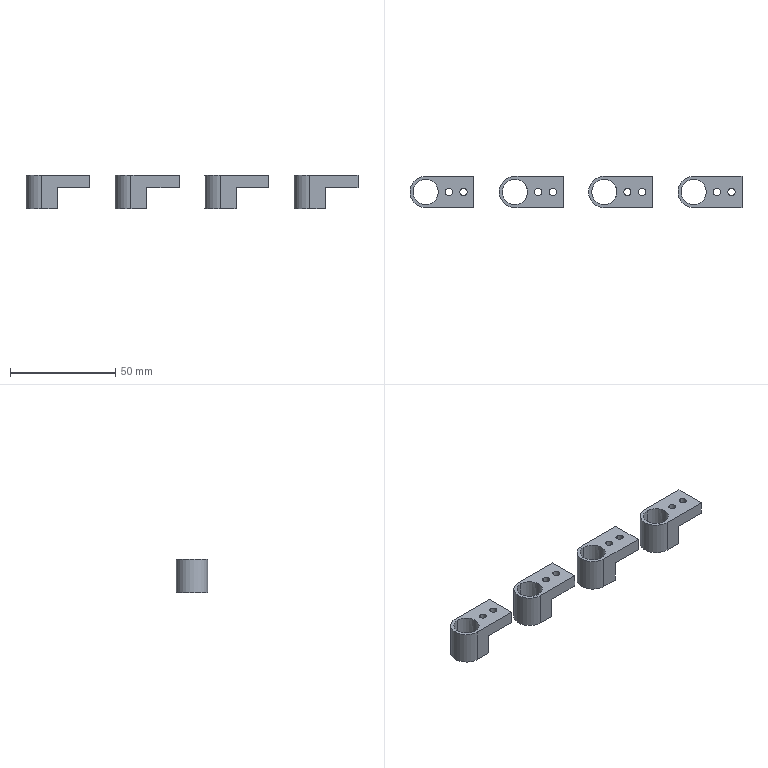NC program | NX | posted with a generic post | part box 158 x 15 x 16 mm
Whole program:
N10 G17 G21 G94 G90
(FLOOR_WALL_COPY , TOOL : D63)
N12 T03 M6
N14 G54
N16 G17 G0 G90 X-34.5 Y0. S6500 M3
N18 G43 Z30. H3
N20 Z6.
N22 G94 G1 Z3. F1500.
N24 X-31.5
N26 X189.5
N28 X192.5
N30 Z6.
N32 G0 Z30.
N34 X-34.5
N36 Z5.
N38 G1 Z2.
N40 X-31.5
N42 X189.5
N44 X192.5
N46 Z5.
N48 G0 Z30.
N50 X-34.5
N52 Z4.
N54 G1 Z1.
N56 X-31.5
N58 X189.5
N60 X192.5
N62 Z4.
N64 G0 Z30.
N66 X-34.5
N68 Z3.
N70 G1 Z0.
N72 X-31.5
N74 X189.5
N76 X192.5
N78 Z3.
N80 G0 Z30.
N82 M5
(FLOOR_WALL_1 , TOOL : D10)
N84 T04 M6
N86 G54
N88 G17 G0 G90 X-4.7 Y-16. S7500 M3
N90 G43 Z30. H4
N92 Z-6.9
N94 G94 G1 Z-9.9 F1000.
N96 Y-13.
N98 Y13. F2500.
N100 X-3.908
N102 Y-13.
N104 X-3.116
N106 Y13.
N108 X-2.324
N110 Y-13.
N112 X-1.532
N114 Y13.
N116 X-0.739
N118 Y-13.
N120 X0.053
N122 Y13.
N124 X0.845
N126 Y-13.
N128 X1.637
N130 Y13.
N132 X2.429
N134 Y-13.
N136 X3.221
N138 Y13.
N140 X4.013
N142 Y-13.
N144 X4.805
N146 Y13.
N148 X5.597
N150 Y-13.
N152 X6.389
N154 Y13.
N156 X7.182
N158 Y-13.
N160 X7.974
N162 Y13.
N164 X8.766
N166 Y-13.
N168 X9.558
N170 Y13.
N172 X10.35
N174 Y-13.
N176 Y-16.
N178 Z-6.9
N180 G0 Z30.
N182 X37.8
N184 Z-6.9
N186 G1 Z-9.9 F1000.
N188 Y-13.
N190 Y13. F2500.
N192 X38.592
N194 Y-13.
N196 X39.384
N198 Y13.
N200 X40.176
N202 Y-13.
N204 X40.968
N206 Y13.
N208 X41.761
N210 Y-13.
N212 X42.553
N214 Y13.
N216 X43.345
N218 Y-13.
N220 X44.137
N222 Y13.
N224 X44.929
N226 Y-13.
N228 X45.721
N230 Y13.
N232 X46.513
N234 Y-13.
N236 X47.305
N238 Y13.
N240 X48.097
N242 Y-13.
N244 X48.889
N246 Y13.
N248 X49.682
N250 Y-13.
N252 X50.474
N254 Y13.
N256 X51.266
N258 Y-13.
N260 X52.058
N262 Y13.
N264 X52.85
N266 Y-13.
N268 Y-16.
N270 Z-6.9
N272 G0 Z30.
N274 X80.3
N276 Z-6.9
N278 G1 Z-9.9 F1000.
N280 Y-13.
N282 Y13. F2500.
N284 X81.092
N286 Y-13.
N288 X81.884
N290 Y13.
N292 X82.676
N294 Y-13.
N296 X83.468
N298 Y13.
N300 X84.261
N302 Y-13.
N304 X85.053
N306 Y13.
N308 X85.845
N310 Y-13.
N312 X86.637
N314 Y13.
N316 X87.429
N318 Y-13.
N320 X88.221
N322 Y13.
N324 X89.013
N326 Y-13.
N328 X89.805
N330 Y13.
N332 X90.597
N334 Y-13.
N336 X91.389
N338 Y13.
N340 X92.182
N342 Y-13.
N344 X92.974
N346 Y13.
N348 X93.766
N350 Y-13.
N352 X94.558
N354 Y13.
N356 X95.35
N358 Y-13.
N360 Y-16.
N362 Z-6.9
N364 G0 Z30.
N366 X122.8
N368 Z-6.9
N370 G1 Z-9.9 F1000.
N372 Y-13.
N374 Y13. F2500.
N376 X123.592
N378 Y-13.
N380 X124.384
N382 Y13.
N384 X125.176
N386 Y-13.
N388 X125.968
N390 Y13.
N392 X126.761
N394 Y-13.
N396 X127.553
N398 Y13.
N400 X128.345
N402 Y-13.
N404 X129.137
N406 Y13.
N408 X129.929
N410 Y-13.
N412 X130.721
N414 Y13.
N416 X131.513
N418 Y-13.
N420 X132.305
N422 Y13.
N424 X133.097
N426 Y-13.
N428 X133.889
N430 Y13.
N432 X134.682
N434 Y-13.
N436 X135.474
N438 Y13.
N440 X136.266
N442 Y-13.
N444 X137.058
N446 Y13.
N448 X137.85
N450 Y-13.
N452 Y-16.
N454 Z-6.9
N456 G0 Z30.
N458 M5
(FLOOR_WALL_1_COPY , TOOL : D10JING)
N460 T14 M6
N462 G54
N464 G17 G0 G90 X0.003 Y-15.5 S7500 M3
N466 G43 Z30. H14
N468 Z-7.
N470 G94 G1 Z-10. F1000.
N472 Y-12.5
N474 Y12.5 F1200.
N476 X5.001
N478 Y-12.5
N480 X10.
N482 Y12.5
N484 Y15.5
N486 Z-7.
N488 G0 Z30.
N490 X10.5 Y-15.5
N492 Z-7.
N494 G1 Z-10. F1000.
N496 Y-12.5
N498 Y12.5 F1200.
N500 Y15.5
N502 Z-7.
N504 G0 Z30.
N506 X42.503 Y-15.5
N508 Z-7.
N510 G1 Z-10. F1000.
N512 Y-12.5
N514 Y12.5 F1200.
N516 X47.501
N518 Y-12.5
N520 X52.5
N522 Y12.5
N524 Y15.5
N526 Z-7.
N528 G0 Z30.
N530 X53. Y-15.5
N532 Z-7.
N534 G1 Z-10. F1000.
N536 Y-12.5
N538 Y12.5 F1200.
N540 Y15.5
N542 Z-7.
N544 G0 Z30.
N546 X85.003 Y-15.5
N548 Z-7.
N550 G1 Z-10. F1000.
N552 Y-12.5
N554 Y12.5 F1200.
N556 X90.001
N558 Y-12.5
N560 X95.
N562 Y12.5
N564 Y15.5
N566 Z-7.
N568 G0 Z30.
N570 X95.5 Y-15.5
N572 Z-7.
N574 G1 Z-10. F1000.
N576 Y-12.5
N578 Y12.5 F1200.
N580 Y15.5
N582 Z-7.
N584 G0 Z30.
N586 X127.503 Y-15.5
N588 Z-7.
N590 G1 Z-10. F1000.
N592 Y-12.5
N594 Y12.5 F1200.
N596 X132.501
N598 Y-12.5
N600 X137.5
N602 Y12.5
N604 Y15.5
N606 Z-7.
N608 G0 Z30.
N610 X138. Y-15.5
N612 Z-7.
N614 G1 Z-10. F1000.
N616 Y-12.5
N618 Y12.5 F1200.
N620 Y15.5
N622 Z-7.
N624 G0 Z30.
N626 M5
(ZLEVEL_PROFILE_2 , TOOL : D6A45)
N628 T01 M6
N630 G54
N632 G17 G0 G90 X152.138 Y2.994 S7500 M3
N634 G43 Z30. H1
N636 Z1.571
N638 G94 G1 Z-1.429 F1250.
N640 X150.96 Y4.399
N642 G3 X150.5 Y4.613 R0.6
N644 X145.887 Y0. R4.613
N646 X150.5 Y4.613 R-4.613
N648 X150.04 Y4.399 R0.6
N650 G1 X148.862 Y2.994
N652 Z1.571
N654 G0 Z30.
N656 X106.362 Y-2.994
N658 Z1.571
N660 G1 Z-1.429
N662 X107.54 Y-4.399
N664 G3 X108. Y-4.613 R0.6
N666 X112.613 Y0. R4.613
N668 X108. Y-4.613 R-4.613
N670 X108.46 Y-4.399 R0.6
N672 G1 X109.638 Y-2.994
N674 Z1.571
N676 G0 Z30.
N678 X63.862
N680 Z1.571
N682 G1 Z-1.429
N684 X65.04 Y-4.399
N686 G3 X65.5 Y-4.613 R0.6
N688 X70.113 Y0. R4.613
N690 X65.5 Y-4.613 R-4.613
N692 X65.96 Y-4.399 R0.6
N694 G1 X67.138 Y-2.994
N696 Z1.571
N698 G0 Z30.
N700 X24.638 Y2.994
N702 Z1.571
N704 G1 Z-1.429
N706 X23.46 Y4.399
N708 G3 X23. Y4.613 R0.6
N710 X18.387 Y0. R4.613
N712 X23. Y4.613 R-4.613
N714 X22.54 Y4.399 R0.6
N716 G1 X21.362 Y2.994
N718 Z1.571
N720 G0 Z30.
N722 X12.913 Y-1.287
N724 Z1.571
N726 G1 Z-1.429
N728 X13.899 Y-0.46
N730 G3 X14.113 Y0. R0.6
N732 G1 Y7.503
N734 G2 X15.497 Y8.887 R1.384
N736 G1 X23.
N738 G2 X31.887 Y0. R8.887
N740 X23. Y-8.887 R8.887
N742 G1 X15.497
N744 G2 X14.113 Y-7.503 R1.384
N746 G1 Y0.
N748 G3 X13.899 Y0.46 R0.6
N750 G1 X12.913 Y1.287
N752 Z1.571
N754 G0 Z30.
N756 X55.413 Y-1.287
N758 Z1.571
N760 G1 Z-1.429
N762 X56.399 Y-0.46
N764 G3 X56.613 Y0. R0.6
N766 G1 Y7.503
N768 G2 X57.997 Y8.887 R1.395
N770 G1 X65.5
N772 G2 X74.387 Y0. R8.887
N774 X65.5 Y-8.887 R8.887
N776 G1 X57.997
N778 G2 X56.613 Y-7.503 R1.395
N780 G1 Y0.
N782 G3 X56.399 Y0.46 R0.6
N784 G1 X55.413 Y1.287
N786 Z1.571
N788 G0 Z30.
N790 X97.913 Y-1.287
N792 Z1.571
N794 G1 Z-1.429
N796 X98.899 Y-0.46
N798 G3 X99.113 Y0. R0.6
N800 G1 Y7.503
N802 G2 X100.497 Y8.887 R1.384
N804 G1 X108.
N806 G2 X116.887 Y0. R8.887
N808 X108. Y-8.887 R8.887
N810 G1 X100.497
N812 G2 X99.113 Y-7.503 R1.384
N814 G1 Y0.
N816 G3 X98.899 Y0.46 R0.6
N818 G1 X97.913 Y1.287
N820 Z1.571
N822 G0 Z30.
N824 X140.413 Y-1.287
N826 Z1.571
N828 G1 Z-1.429
N830 X141.399 Y-0.46
N832 G3 X141.613 Y0. R0.6
N834 G1 Y7.503
N836 G2 X142.997 Y8.887 R1.384
N838 G1 X150.5
N840 G2 X159.387 Y0. R8.887
N842 X150.5 Y-8.887 R8.887
N844 G1 X142.997
N846 G2 X141.613 Y-7.503 R1.384
N848 G1 Y0.
N850 G3 X141.399 Y0.46 R0.6
N852 G1 X140.413 Y1.287
N854 Z1.571
N856 G0 Z30.
(ZLEVEL_PROFILE_2_COPY , TOOL : D6A45)
N858 X96.971 Y0.741
N860 Z-7.
N862 G1 Z-11.
N864 G3 X96.971 Y-0.741 R0.741
N866 X97.204 Y-0.643 R0.3
N868 G1 Z-8.
N870 G0 Z30.
N872 X90. Y0.741
N874 Z-7.
N876 G1 Z-11.
N878 G3 X89.259 Y0. R0.741
N880 X90. Y0.741 R-0.741
N882 X89.54 Y0.527 R0.6
N884 G1 Z-8.
N886 G0 Z30.
N888 X11.983 Y0.741
N890 Z-7.
N892 G1 Z-11.
N894 G3 X11.983 Y-0.741 R0.741
N896 X12.215 Y-0.639 R0.3
N898 G1 Z-8.
N900 G0 Z30.
N902 X4.259 Y0.
N904 Z-7.
N906 G1 Z-11.
N908 G3 X5. Y-0.741 R0.741
N910 X4.259 Y0. R-0.741
N912 X4.473 Y-0.46 R0.6
N914 G1 Z-8.
N916 G0 Z30.
N918 X132.5 Y0.741
N920 Z-7.
N922 G1 Z-11.
N924 X132.498
N926 G3 X131.759 Y-0.002 R0.741
N928 X132.5 Y0.741 R-0.741
N930 X132.04 Y0.527 R0.6
N932 G1 Z-8.
N934 G0 Z30.
N936 X139.476 Y0.741
N938 Z-7.
N940 G1 Z-11.
N942 G3 X139.476 Y-0.741 R0.741
N944 X139.709 Y-0.641 R0.3
N946 G1 Z-8.
N948 G0 Z30.
N950 X54.483 Y0.741
N952 Z-7.
N954 G1 Z-11.
N956 G3 X54.472 Y-0.741 R0.741
N958 X54.706 Y-0.642 R0.3
N960 G1 Z-8.
N962 G0 Z30.
N964 X47.5 Y0.741
N966 Z-7.
N968 G1 Z-11.
N970 X47.491
N972 G3 X47.5 Y0.741 R-0.741
N974 X47.04 Y0.527 R0.6
N976 G1 Z-8.
N978 G0 Z30.
N980 X54.514 Y-9.659
N982 Z-8.
N984 G1 Z-11.
N986 X54.834 Y-8.566
N988 G3 X54.605 Y-8.459 R0.3
N990 G1 X42.497
N992 G2 X41.541 Y-7.503 R0.956
N994 G1 Y7.503
N996 G2 X42.497 Y8.459 R0.956
N998 G1 X54.605
N1000 G3 X54.834 Y8.566 R0.3
N1002 G1 X54.514 Y9.659
N1004 Z-8.
N1006 G0 Z30.
N1008 X139.514 Y-9.659
N1010 Z-8.
N1012 G1 Z-11.
N1014 X139.837 Y-8.566
N1016 G3 X139.607 Y-8.459 R0.3
N1018 G1 X127.497
N1020 G2 X126.541 Y-7.503 R0.956
N1022 G1 Y7.503
N1024 G2 X127.497 Y8.459 R0.956
N1026 G1 X139.607
N1028 G3 X139.837 Y8.566 R0.3
N1030 G1 X139.514 Y9.659
N1032 Z-8.
N1034 G0 Z30.
N1036 X12.014 Y-9.659
N1038 Z-8.
N1040 G1 Z-11.
N1042 X12.349 Y-8.566
N1044 G3 X12.119 Y-8.459 R0.3
N1046 G1 X-0.003
N1048 G2 X-0.959 Y-7.503 R0.99
N1050 G1 Y7.503
N1052 G2 X-0.003 Y8.459 R0.99
N1054 G1 X12.119
N1056 G3 X12.349 Y8.566 R0.3
N1058 G1 X12.014 Y9.659
N1060 Z-8.
N1062 G0 Z30.
N1064 X97.014 Y-9.659
N1066 Z-8.
N1068 G1 Z-11.
N1070 X97.344 Y-8.566
N1072 G3 X97.114 Y-8.459 R0.3
N1074 G1 X84.997
N1076 G2 X84.041 Y-7.503 R0.98
N1078 G1 Y7.503
N1080 G2 X84.997 Y8.459 R0.98
N1082 G1 X97.114
N1084 G3 X97.344 Y8.566 R0.3
N1086 G1 X97.014 Y9.659
N1088 Z-8.
N1090 G0 Z30.
N1092 M5
N1094 M2